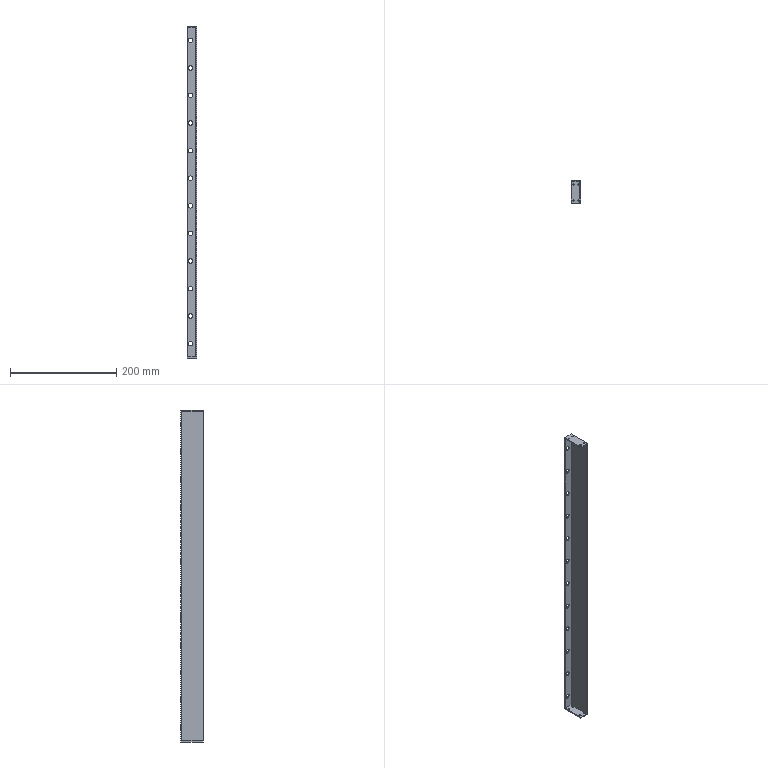Part | STEP file | Storage prox plate | 1 solid | 50 faces | box 17 x 43 x 626 mm | volume 73636 mm3 | cylinder 40 | plane 10 | commonest cylinder face diameters 8.5 x24 2.5 x16